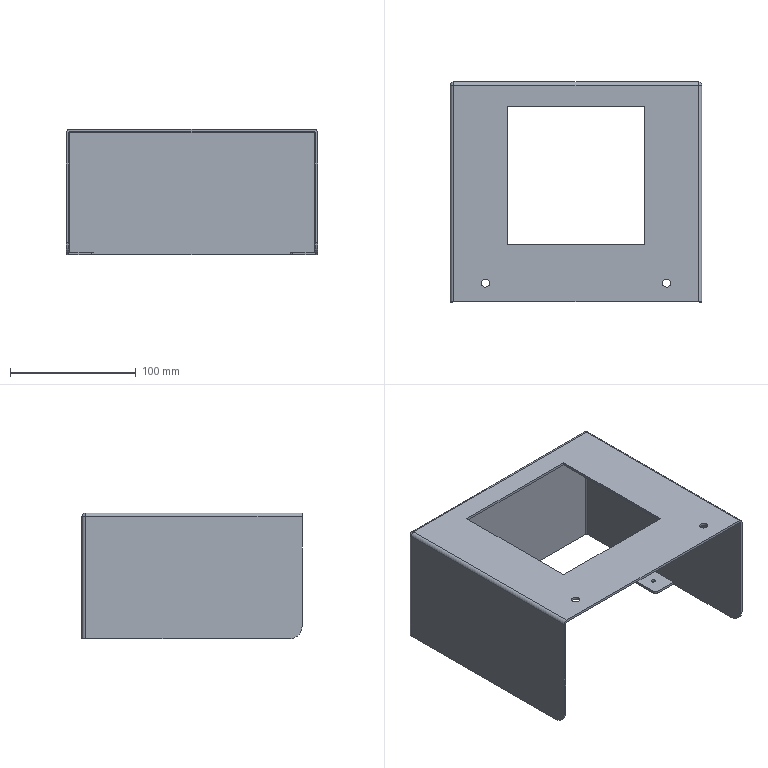Part | STEP file | ND25021-01-JDKM-04-BJ | 1 solid | 50 faces | box 200 x 175 x 100 mm | volume 153713 mm3 | cylinder 24 | plane 22 | sphere 4 | commonest cylinder face diameters 2 x5 6 x5 3.3 x4 4 x4 6.5 x4 20 x2